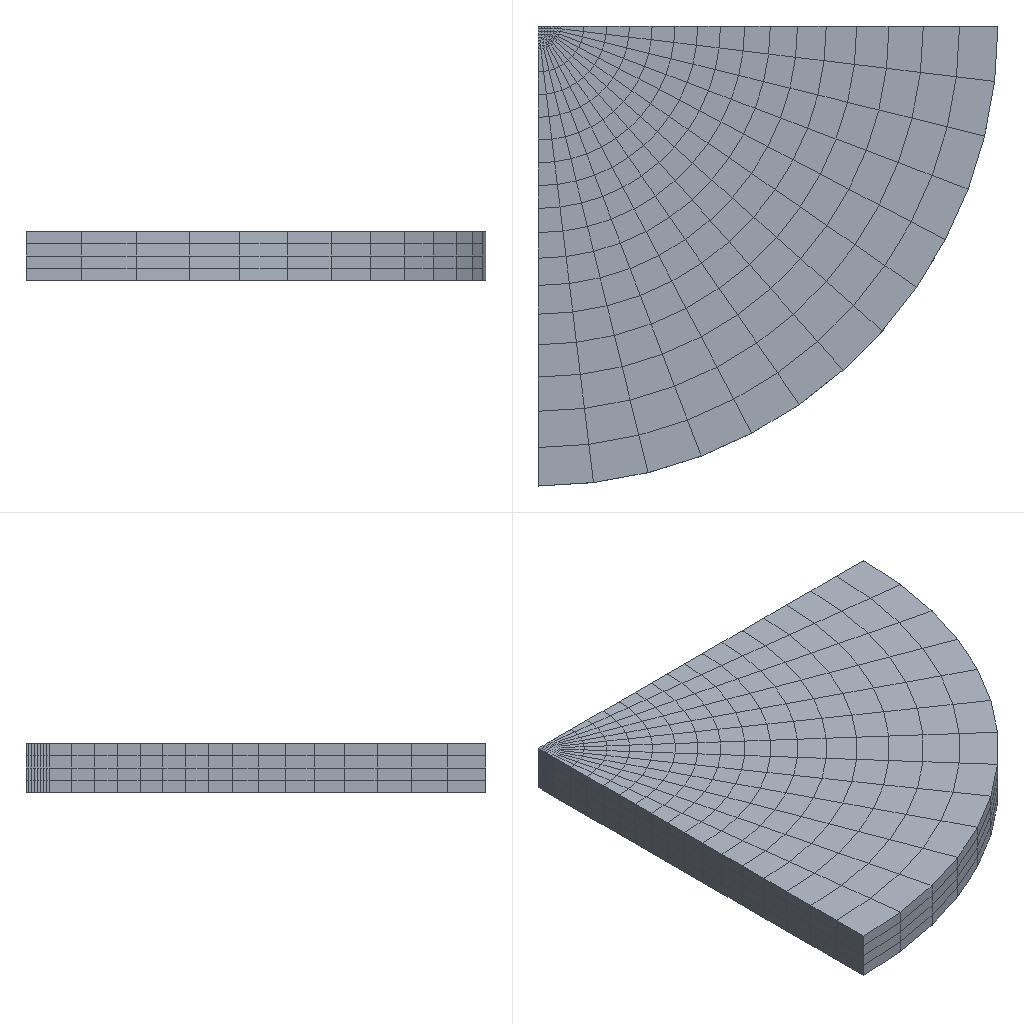Simulation study | abaqus
Set-up summary:
category,name,step,type,value,unit,region
solver,abaqus
solver,version,,,Abaqus/Standard 3DEXPERIENCE R2017x
units,not stated in the deck,,not stated
analysis,deck,,static,static
load_step,Step-1,Step-1,static
load_step,Step-2,Step-2,transient
load_step,requested,,,2
mesh,nodes,,,1795
mesh,elements,,,1319
element_type,R3D3,,rigid,4
element_type,R3D4,,rigid,263
element_type,C3D8R,,solid,1052
load,load commands in deck,,count,2
bc,support commands in deck,,count,19
material,MATERIAL-1,,in results
check,setup vs results,,match,"per instance, exact: element labels, types and connectivity; labels of the nodes the elements use; coordinates of those nodes at SINGLE_PRECISION in 2 of 4 instance(s)"
Abaqus input file, long lists of numbers shortened:
*Heading
** Job name: Job-1 Model name: Standard
** Generated by: Abaqus/CAE 2017
*Preprint, echo=NO, model=NO, history=NO, contact=NO
**
** PARTS
**
*Part, name=ball
*End Part
**
*Part, name=die
*End Part
**
*Part, name=holder
*End Part
**
*Part, name=specimen
*End Part
**
**
** ASSEMBLY
**
*Assembly, name=Assembly
**
*Instance, name=specimen-1, part=specimen
*Node
      1,           0., -0.2,           0.
      2,  0.2,           0.,           0.
** (1468 more lines like these left out)
*Element, type=C3D8R
  1,   88,  340,  841,  310,    1,   15,  190,   48
  2,  340,  341,  842,  841,   15,   16,  191,  190
** (1050 more lines like these left out)
*Nset, nset=Set-1, generate
    1,  1470,     1
*Elset, elset=Set-1, generate
    1,  1052,     1
*Nset, nset=Set-3, generate
    1,  1470,     1
*Elset, elset=Set-3, generate
    1,  1052,     1
*Elset, elset=_specimen-up_S1, internal
  235,  236,  237,  238,  239,  240,  241,  242,  243,  244,  245,  246,  247,  248,  249,  250
  251,  252,  253,  254,  255,  256,  257,  258,  259,  260,  261,  262,  263,  264,  265,  266
** (11 more lines like these left out)
*Elset, elset=_specimen-up_S3, internal
 423, 424, 425, 426, 427, 428, 449, 450, 451, 452, 453, 454, 455, 463, 464, 465
 466, 467, 468, 469, 477, 478, 479, 480, 481, 482, 483, 491, 492, 493, 494, 495
** (1 more lines like these left out)
*Elset, elset=_specimen-up_S4, internal, generate
 436,  448,    2
*Surface, type=ELEMENT, name=specimen-up
_specimen-up_S1, S1
_specimen-up_S3, S3
_specimen-up_S4, S4
*Elset, elset=_specimen-lower_S2, internal
   1,   2,   3,   4,   5,   6,   7,   8,   9,  10,  11,  12,  13,  14,  15,  16
  17,  18,  19,  20,  21,  22,  23,  24,  25,  26,  27,  28,  29,  30,  31,  32
** (15 more lines like these left out)
*Surface, type=ELEMENT, name=specimen-lower
_specimen-lower_S2, S2
*Orientation, name=Ori-10
          1.,           0.,           0.,           0.,           1.,           0.
1, 0.
** Section: Section-1
*Solid Section, elset=Set-3, orientation=Ori-10, material=Material-1
,
*End Instance
**
*Instance, name=die-1, part=die
 8.88178419700125e-16,           0.,           0.
 8.88178419700125e-16,           0.,           0.,           1.,           0.,           0.,          90.
*Node
      1,           0.,  -1.2,           2.
      2,           0., -0.2,           2.
** (152 more lines like these left out)
*Element, type=R3D4
 1,   1,   9,  71,  38
 2,   9,  10,  72,  71
** (128 more lines like these left out)
*Node
    155,    2.263,  1.09925615e-14,    2.263
*Nset, nset=die-1-RefPt_, internal
155,
*Elset, elset=_die_SPOS, internal, generate
   1,  130,    1
*Surface, type=ELEMENT, name=die
_die_SPOS, SPOS
*Elset, elset=die-1, generate
   1,  130,    1
*End Instance
**
*Instance, name=holder-1, part=holder
          0.,           0.,         0.42
          0.,           0.,         0.42,           1.,           0.,         0.42,          90.
*Node
      1,           0.,          1.5,         1.25
      2,           0.,           0.,         1.25
** (62 more lines like these left out)
*Element, type=R3D4
 1,  1,  7, 33, 16
 2,  7,  8, 34, 33
** (46 more lines like these left out)
*Element, type=R3D3
13, 57, 45, 43
*Node
     65,   2.298,  3.42011724e-15,   2.298
*Nset, nset=holder-1-RefPt_, internal
65,
*Elset, elset=_holder_SNEG, internal, generate
 13,  49,   1
*Surface, type=ELEMENT, name=holder
_holder_SNEG, SNEG
*Elset, elset=_hold-2_SNEG, internal, generate
  1,  12,   1
*Surface, type=ELEMENT, name=hold-2
_hold-2_SNEG, SNEG
*Elset, elset=holder-1, generate
  1,  49,   1
*End Instance
**
*Instance, name=ball-1, part=ball
          0.,  -8.32667268468867e-16,       -13.33
          0.,  -8.32667268468867e-16,       -13.33,           1.,  -8.32667268468867e-16,       -13.33,          90.
*Node
      1,           0.,    13.763,  0.1779
      2,           0.,   13.863,  0.5193
** (102 more lines like these left out)
*Element, type=R3D3
1, 75, 74, 71
2, 52, 51, 64
** (1 more lines like these left out)
*Element, type=R3D4
 4,  25,  24,   8,   1
 5,  78,  98,  77,  68
** (83 more lines like these left out)
*Node
    105,  7.6540425e-17,          15.,         1.25
*Nset, nset=ball-1-RefPt_, internal
105,
*Elset, elset=_ball_SNEG, internal, generate
  1,  88,   1
*Surface, type=ELEMENT, name=ball
_ball_SNEG, SNEG
*Elset, elset=ball-1, generate
  1,  88,   1
*End Instance
**
*Nset, nset=RP, instance=ball-1
 105,
*Nset, nset=Set-292, instance=ball-1
 105,
*Nset, nset=Set-293, instance=specimen-1
   2,   3,   5,   6,   9,  10,  11,  13,  27,  28,  29,  30,  31,  61,  62,  63
  64,  65,  89,  90,  91,  92,  93,  94,  95,  96,  97,  98,  99, 100, 108, 109
** (6 more lines like these left out)
*Elset, elset=Set-293, instance=specimen-1
   13,   26,   39,   52,   65,   78,   91,  104,  117,  130,  143,  156,  169,  182,  195,  208
  221,  234,  247,  260,  273,  286,  299,  312,  313,  320,  345,  352,  359,  366,  373,  380
** (4 more lines like these left out)
*Nset, nset=Set-294, instance=specimen-1
   1,   4,   7,   8,   9,  10,  12,  14,  44,  45,  46,  47,  48,  78,  79,  80
  81,  82,  83,  84,  85,  86,  87,  88, 101, 102, 103, 104, 105, 106, 107, 108
** (6 more lines like these left out)
*Elset, elset=Set-294, instance=specimen-1
    1,   14,   27,   40,   53,   66,   79,   92,  105,  118,  131,  144,  157,  170,  183,  196
  209,  222,  235,  248,  261,  274,  287,  300,  332,  338,  339,  340,  341,  342,  343,  344
** (4 more lines like these left out)
*Nset, nset=Set-295, instance=ball-1
 105,
*Nset, nset=Set-296, instance=die-1
 155,
*Nset, nset=Set-297, instance=holder-1
 65,
*Rigid Body, ref node=die-1.die-1-RefPt_, elset=die-1.die-1
*Rigid Body, ref node=holder-1.holder-1-RefPt_, elset=holder-1.holder-1
*Rigid Body, ref node=ball-1.ball-1-RefPt_, elset=ball-1.ball-1
*End Assembly
*Amplitude, name=Amp-2, time=TOTAL TIME
             0.,              0.,              1.,              1.
**
** MATERIALS
**
*Material, name=Material-1
*Creep
 4.8e-15, 5.75,   0.
*Potential
1.,      0.8,      0.8,     0.86,     0.86, 0.7397
*Elastic
36000., 0.3
*Plastic
320.,0.
**
** INTERACTION PROPERTIES
**
*Surface Interaction, name=specimen_ball
1.,
*Friction, slip tolerance=0.005
 0.2,
*Surface Behavior, pressure-overclosure=HARD
*Surface Interaction, name=specimen_die
1.,
*Friction, slip tolerance=0.005
 0.2,
*Surface Behavior, pressure-overclosure=HARD
*Surface Interaction, name=specimen_holder
1.,
*Friction, slip tolerance=0.005
 0.2,
*Surface Behavior, pressure-overclosure=HARD
**
** BOUNDARY CONDITIONS
**
** Name: BC-5 Type: 对称/反对称/完全固定
*Boundary
Set-293, YSYMM
** Name: BC-7 Type: 对称/反对称/完全固定
*Boundary
Set-294, XSYMM
** Name: bc_ball_xz Type: Displacement/Rotation
*Boundary
Set-295, 1, 1
Set-295, 2, 2
Set-295, 4, 4
Set-295, 5, 5
Set-295, 6, 6
** Name: bc_die Type: Displacement/Rotation
*Boundary
Set-296, 1, 1
Set-296, 2, 2
Set-296, 3, 3
Set-296, 4, 4
Set-296, 5, 5
Set-296, 6, 6
** Name: bc_holder Type: Displacement/Rotation
*Boundary
Set-297, 1, 1
Set-297, 2, 2
Set-297, 3, 3
Set-297, 4, 4
Set-297, 5, 5
Set-297, 6, 6
**
** INTERACTIONS
**
** Interaction: Int-1
*Contact Pair, interaction=specimen_ball, type=SURFACE TO SURFACE, adjust=0.0
specimen-1.specimen-up, ball-1.ball
** Interaction: Int-2
*Contact Pair, interaction=specimen_holder, type=SURFACE TO SURFACE, adjust=0.0
specimen-1.specimen-up, holder-1.holder
** Interaction: Int-3
*Contact Pair, interaction=specimen_die, type=SURFACE TO SURFACE, adjust=0.0
specimen-1.specimen-lower, die-1.die
** ----------------------------------------------------------------
**
** STEP: Step-1
**
*Step, name=Step-1, nlgeom=YES, inc=1000
*Static, stabilize=0.0002, allsdtol=0.05, continue=NO
1e-08, 1e-06, 1e-11, 1e-06
**
** LOADS
**
** Name: Load-1   Type: Concentrated force
*Cload
Set-292, 2, 0.
Set-292, 3, -25.
**
** OUTPUT REQUESTS
**
*Restart, write, frequency=0
**
** FIELD OUTPUT: F-Output-1
**
*Output, field
*Node Output
CF, RF, RM, RT, U, V
*Element Output, directions=YES
E, LE, MISES, MISESMAX, MISESONLY, PE, PEEQ, PEEQT, PEMAG, S, SF, SSAVG, TSHR
*Contact Output
CDISP, CSTRESS
**
** HISTORY OUTPUT: H-Output-2
**
*Output, history
*Node Output, nset=RP
RF3, U3
**
** HISTORY OUTPUT: H-Output-1
**
*Output, history, variable=PRESELECT
*End Step
** ----------------------------------------------------------------
**
** STEP: Step-2
**
*Step, name=Step-2, nlgeom=YES, inc=5000
*Visco, cetol=1., creep=EXPLICIT, stabilize=0.0002, allsdtol=0.05, continue=NO
1., 1e+06, 1e-56, 1e+06
**
** CONTROLS
**
*Controls, reset
*Controls, parameters=time incrementation
, , , , , , , 50, , ,
**
** SOLVER CONTROLS
**
*Solver Controls, reset
*Solver Controls
,
**
** OUTPUT REQUESTS
**
*Restart, write, frequency=0
**
** FIELD OUTPUT: F-Output-1
**
*Output, field
*Node Output
CF, RF, U
*Element Output, directions=YES
CE, CEEQ, E, LE, PE, PEEQ, PEMAG, S
*Contact Output
CDISP, CSTRESS
**
** HISTORY OUTPUT: H-Output-2
**
*Output, history
*Node Output, nset=RP
RF3, U3
**
** HISTORY OUTPUT: H-Output-1
**
*Output, history, variable=PRESELECT
*End Step
Results summary:
result,step,,completed,increments=32 time=1e-06/1e-06
result,step,,partial,increments=1299 time=8151.857/1000000.0
result,analysis,,,transient
result,last_loadstep,,,2
result,primary field,,,U
result,reaction total,,FX,-1.783,model units
result,reaction total,,FY,1.878,model units
result,reaction total,,FZ,-1.478,model units